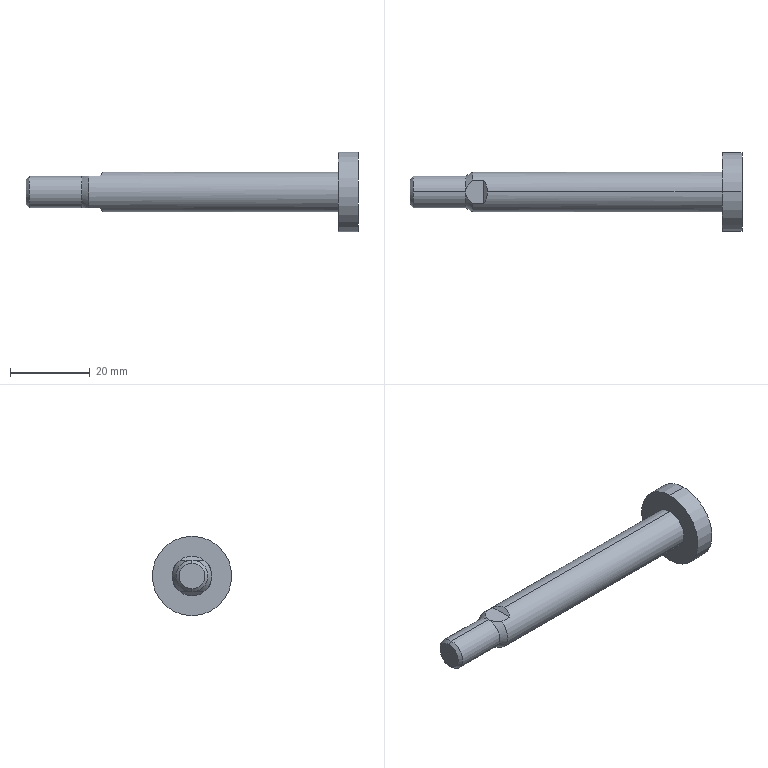Part | SolidWorks | features BaseBody 1 | 1 solid | 17 faces | box 83.5 x 20 x 20 mm | volume 7277 mm3 | plane 7 | cylinder 6 | cone 4 | commonest cylinder face diameters 8 x2 10 x2 20 x2
STEP:
#1=CARTESIAN_POINT('',(0.,3.,4.));
#2=VERTEX_POINT('',#1);
#3=CARTESIAN_POINT('',(1.,0.,5.));
#4=VERTEX_POINT('',#3);
#5=CARTESIAN_POINT('',(0.,3.,4.));
#6=CARTESIAN_POINT('',(0.6549,2.127,4.655));
#7=CARTESIAN_POINT('',(1.,1.091,5.));
#8=CARTESIAN_POINT('',(1.,0.,5.));
#9=(BOUNDED_CURVE()B_SPLINE_CURVE(3,(#5,#6,#7,#8),.UNSPECIFIED.,.F.,.T.)B_SPLINE_CURVE_WITH_KNOTS((4,4),(5.64,6.283),.UNSPECIFIED.)CURVE()GEOMETRIC_REPRESENTATION_ITEM()RATIONAL_B_SPLINE_CURVE((1.,0.9658,0.9658,1.))REPRESENTATION_ITEM(''));
#10=EDGE_CURVE('',#2,#4,#9,.T.);
#11=ORIENTED_EDGE('',*,*,#10,.T.);
#12=CARTESIAN_POINT('',(60.,0.,5.));
#13=VERTEX_POINT('',#12);
#14=CARTESIAN_POINT('',(28.616,0.,5.));
#15=DIRECTION('',(1.,0.,0.));
#16=VECTOR('',#15,1000.);
#17=LINE('',#14,#16);
#18=EDGE_CURVE('',#4,#13,#17,.T.);
#19=ORIENTED_EDGE('',*,*,#18,.T.);
#20=CARTESIAN_POINT('',(60.,0.,-5.));
#21=VERTEX_POINT('',#20);
#22=CARTESIAN_POINT('',(60.,0.,0.));
#23=DIRECTION('',(-1.,0.,0.));
#24=DIRECTION('',(0.,0.,-1.));
#25=AXIS2_PLACEMENT_3D('',#22,#23,#24);
#26=CIRCLE('',#25,5.);
#27=EDGE_CURVE('',#13,#21,#26,.T.);
#28=ORIENTED_EDGE('',*,*,#27,.T.);
#29=CARTESIAN_POINT('',(1.,0.,-5.));
#30=VERTEX_POINT('',#29);
#31=CARTESIAN_POINT('',(28.616,0.,-5.));
#32=DIRECTION('',(1.,0.,0.));
#33=VECTOR('',#32,1000.);
#34=LINE('',#31,#33);
#35=EDGE_CURVE('',#30,#21,#34,.T.);
#36=ORIENTED_EDGE('',*,*,#35,.F.);
#37=CARTESIAN_POINT('',(0.,3.,-4.));
#38=VERTEX_POINT('',#37);
#39=CARTESIAN_POINT('',(1.,0.,-5.));
#40=CARTESIAN_POINT('',(1.,1.091,-5.));
#41=CARTESIAN_POINT('',(0.6549,2.127,-4.655));
#42=CARTESIAN_POINT('',(0.,3.,-4.));
#43=(BOUNDED_CURVE()B_SPLINE_CURVE(3,(#39,#40,#41,#42),.UNSPECIFIED.,.F.,.T.)B_SPLINE_CURVE_WITH_KNOTS((4,4),(0.,0.6435),.UNSPECIFIED.)CURVE()GEOMETRIC_REPRESENTATION_ITEM()RATIONAL_B_SPLINE_CURVE((1.,0.9658,0.9658,1.))REPRESENTATION_ITEM(''));
#44=EDGE_CURVE('',#30,#38,#43,.T.);
#45=ORIENTED_EDGE('',*,*,#44,.T.);
#46=CARTESIAN_POINT('',(-2.768,3.,-4.));
#47=VERTEX_POINT('',#46);
#48=CARTESIAN_POINT('',(28.616,3.,-4.));
#49=DIRECTION('',(-1.,0.,0.));
#50=VECTOR('',#49,1000.);
#51=LINE('',#48,#50);
#52=EDGE_CURVE('',#38,#47,#51,.T.);
#53=ORIENTED_EDGE('',*,*,#52,.T.);
#54=CARTESIAN_POINT('',(-2.768,3.,4.));
#55=VERTEX_POINT('',#54);
#56=CARTESIAN_POINT('',(-2.768,0.,0.));
#57=DIRECTION('',(1.,0.,0.));
#58=DIRECTION('',(0.,0.,-1.));
#59=AXIS2_PLACEMENT_3D('',#56,#57,#58);
#60=CIRCLE('',#59,5.);
#61=EDGE_CURVE('',#47,#55,#60,.T.);
#62=ORIENTED_EDGE('',*,*,#61,.T.);
#63=CARTESIAN_POINT('',(28.616,3.,4.));
#64=DIRECTION('',(1.,0.,0.));
#65=VECTOR('',#64,1000.);
#66=LINE('',#63,#65);
#67=EDGE_CURVE('',#55,#2,#66,.T.);
#68=ORIENTED_EDGE('',*,*,#67,.T.);
#69=EDGE_LOOP('',(#11,#19,#28,#36,#45,#53,#62,#68));
#70=FACE_OUTER_BOUND('',#69,.T.);
#71=CARTESIAN_POINT('',(28.616,0.,0.));
#72=DIRECTION('',(1.,0.,0.));
#73=DIRECTION('',(0.,0.,-1.));
#74=AXIS2_PLACEMENT_3D('',#71,#72,#73);
#75=CYLINDRICAL_SURFACE('',#74,5.);
#76=ADVANCED_FACE('',(#70),#75,.T.);
#77=CARTESIAN_POINT('',(60.,0.,10.));
#78=VERTEX_POINT('',#77);
#79=CARTESIAN_POINT('',(60.,0.,-10.));
#80=VERTEX_POINT('',#79);
#81=CARTESIAN_POINT('',(60.,0.,0.));
#82=DIRECTION('',(-1.,0.,0.));
#83=DIRECTION('',(0.,0.,-1.));
#84=AXIS2_PLACEMENT_3D('',#81,#82,#83);
#85=CIRCLE('',#84,10.);
#86=EDGE_CURVE('',#78,#80,#85,.T.);
#87=ORIENTED_EDGE('',*,*,#86,.F.);
#88=CARTESIAN_POINT('',(65.,0.,10.));
#89=VERTEX_POINT('',#88);
#90=CARTESIAN_POINT('',(62.5,0.,10.));
#91=DIRECTION('',(1.,0.,0.));
#92=VECTOR('',#91,1000.);
#93=LINE('',#90,#92);
#94=EDGE_CURVE('',#78,#89,#93,.T.);
#95=ORIENTED_EDGE('',*,*,#94,.T.);
#96=CARTESIAN_POINT('',(65.,0.,-10.));
#97=VERTEX_POINT('',#96);
#98=CARTESIAN_POINT('',(65.,0.,0.));
#99=DIRECTION('',(-1.,0.,0.));
#100=DIRECTION('',(0.,0.,-1.));
#101=AXIS2_PLACEMENT_3D('',#98,#99,#100);
#102=CIRCLE('',#101,10.);
#103=EDGE_CURVE('',#89,#97,#102,.T.);
#104=ORIENTED_EDGE('',*,*,#103,.T.);
#105=CARTESIAN_POINT('',(62.5,0.,-10.));
#106=DIRECTION('',(1.,0.,0.));
#107=VECTOR('',#106,1000.);
#108=LINE('',#105,#107);
#109=EDGE_CURVE('',#80,#97,#108,.T.);
#110=ORIENTED_EDGE('',*,*,#109,.F.);
#111=EDGE_LOOP('',(#87,#95,#104,#110));
#112=FACE_OUTER_BOUND('',#111,.T.);
#113=CARTESIAN_POINT('',(62.5,0.,0.));
#114=DIRECTION('',(1.,0.,0.));
#115=DIRECTION('',(0.,0.,-1.));
#116=AXIS2_PLACEMENT_3D('',#113,#114,#115);
#117=CYLINDRICAL_SURFACE('',#116,10.);
#118=ADVANCED_FACE('',(#112),#117,.T.);
#119=CARTESIAN_POINT('',(-17.733,0.,-4.));
#120=VERTEX_POINT('',#119);
#121=CARTESIAN_POINT('',(-17.733,0.,4.));
#122=VERTEX_POINT('',#121);
#123=CARTESIAN_POINT('',(-17.733,0.,0.));
#124=DIRECTION('',(1.,0.,0.));
#125=DIRECTION('',(0.,0.,-1.));
#126=AXIS2_PLACEMENT_3D('',#123,#124,#125);
#127=CIRCLE('',#126,4.);
#128=EDGE_CURVE('',#120,#122,#127,.T.);
#129=ORIENTED_EDGE('',*,*,#128,.T.);
#130=CARTESIAN_POINT('',(-4.5,0.,4.));
#131=VERTEX_POINT('',#130);
#132=CARTESIAN_POINT('',(-11.117,0.,4.));
#133=DIRECTION('',(1.,0.,0.));
#134=VECTOR('',#133,1000.);
#135=LINE('',#132,#134);
#136=EDGE_CURVE('',#122,#131,#135,.T.);
#137=ORIENTED_EDGE('',*,*,#136,.T.);
#138=CARTESIAN_POINT('',(-4.5,0.,-4.));
#139=VERTEX_POINT('',#138);
#140=CARTESIAN_POINT('',(-4.5,0.,0.));
#141=DIRECTION('',(1.,0.,0.));
#142=DIRECTION('',(0.,1.,0.));
#143=AXIS2_PLACEMENT_3D('',#140,#141,#142);
#144=CIRCLE('',#143,4.);
#145=EDGE_CURVE('',#139,#131,#144,.T.);
#146=ORIENTED_EDGE('',*,*,#145,.F.);
#147=CARTESIAN_POINT('',(-11.117,0.,-4.));
#148=DIRECTION('',(1.,0.,0.));
#149=VECTOR('',#148,1000.);
#150=LINE('',#147,#149);
#151=EDGE_CURVE('',#120,#139,#150,.T.);
#152=ORIENTED_EDGE('',*,*,#151,.F.);
#153=EDGE_LOOP('',(#129,#137,#146,#152));
#154=FACE_OUTER_BOUND('',#153,.T.);
#155=CARTESIAN_POINT('',(-11.117,0.,0.));
#156=DIRECTION('',(1.,0.,0.));
#157=DIRECTION('',(0.,0.,-1.));
#158=AXIS2_PLACEMENT_3D('',#155,#156,#157);
#159=CYLINDRICAL_SURFACE('',#158,4.);
#160=ADVANCED_FACE('',(#154),#159,.T.);
#161=CARTESIAN_POINT('',(-18.5,0.,-3.233));
#162=VERTEX_POINT('',#161);
#163=CARTESIAN_POINT('',(-18.5,0.,3.233));
#164=VERTEX_POINT('',#163);
#165=CARTESIAN_POINT('',(-18.5,0.,0.));
#166=DIRECTION('',(1.,0.,0.));
#167=DIRECTION('',(0.,0.,-1.));
#168=AXIS2_PLACEMENT_3D('',#165,#166,#167);
#169=CIRCLE('',#168,3.233);
#170=EDGE_CURVE('',#162,#164,#169,.T.);
#171=ORIENTED_EDGE('',*,*,#170,.T.);
#172=CARTESIAN_POINT('',(-17.733,0.,4.));
#173=DIRECTION('',(0.7071,0.,0.7071));
#174=VECTOR('',#173,1000.);
#175=LINE('',#172,#174);
#176=EDGE_CURVE('',#164,#122,#175,.T.);
#177=ORIENTED_EDGE('',*,*,#176,.T.);
#178=ORIENTED_EDGE('',*,*,#128,.F.);
#179=CARTESIAN_POINT('',(-17.733,0.,-4.));
#180=DIRECTION('',(0.7071,0.,-0.7071));
#181=VECTOR('',#180,1000.);
#182=LINE('',#179,#181);
#183=EDGE_CURVE('',#162,#120,#182,.T.);
#184=ORIENTED_EDGE('',*,*,#183,.F.);
#185=EDGE_LOOP('',(#171,#177,#178,#184));
#186=FACE_OUTER_BOUND('',#185,.T.);
#187=CARTESIAN_POINT('',(-17.733,0.,0.));
#188=DIRECTION('',(1.,0.,0.));
#189=DIRECTION('',(0.,0.,-1.));
#190=AXIS2_PLACEMENT_3D('',#187,#188,#189);
#191=CONICAL_SURFACE('',#190,4.,0.7854);
#192=ADVANCED_FACE('',(#186),#191,.T.);
#193=ORIENTED_EDGE('',*,*,#18,.F.);
#194=CARTESIAN_POINT('',(0.,-3.,4.));
#195=VERTEX_POINT('',#194);
#196=CARTESIAN_POINT('',(1.,0.,5.));
#197=CARTESIAN_POINT('',(1.,-1.091,5.));
#198=CARTESIAN_POINT('',(0.6549,-2.127,4.655));
#199=CARTESIAN_POINT('',(0.,-3.,4.));
#200=(BOUNDED_CURVE()B_SPLINE_CURVE(3,(#196,#197,#198,#199),.UNSPECIFIED.,.F.,.T.)B_SPLINE_CURVE_WITH_KNOTS((4,4),(0.,0.6435),.UNSPECIFIED.)CURVE()GEOMETRIC_REPRESENTATION_ITEM()RATIONAL_B_SPLINE_CURVE((1.,0.9658,0.9658,1.))REPRESENTATION_ITEM(''));
#201=EDGE_CURVE('',#4,#195,#200,.T.);
#202=ORIENTED_EDGE('',*,*,#201,.T.);
#203=CARTESIAN_POINT('',(-2.768,-3.,4.));
#204=VERTEX_POINT('',#203);
#205=CARTESIAN_POINT('',(28.616,-3.,4.));
#206=DIRECTION('',(-1.,0.,0.));
#207=VECTOR('',#206,1000.);
#208=LINE('',#205,#207);
#209=EDGE_CURVE('',#195,#204,#208,.T.);
#210=ORIENTED_EDGE('',*,*,#209,.T.);
#211=CARTESIAN_POINT('',(-2.768,-3.,-4.));
#212=VERTEX_POINT('',#211);
#213=CARTESIAN_POINT('',(-2.768,0.,0.));
#214=DIRECTION('',(1.,0.,0.));
#215=DIRECTION('',(0.,0.,-1.));
#216=AXIS2_PLACEMENT_3D('',#213,#214,#215);
#217=CIRCLE('',#216,5.);
#218=EDGE_CURVE('',#204,#212,#217,.T.);
#219=ORIENTED_EDGE('',*,*,#218,.T.);
#220=CARTESIAN_POINT('',(0.,-3.,-4.));
#221=VERTEX_POINT('',#220);
#222=CARTESIAN_POINT('',(28.616,-3.,-4.));
#223=DIRECTION('',(1.,0.,0.));
#224=VECTOR('',#223,1000.);
#225=LINE('',#222,#224);
#226=EDGE_CURVE('',#212,#221,#225,.T.);
#227=ORIENTED_EDGE('',*,*,#226,.T.);
#228=CARTESIAN_POINT('',(0.,-3.,-4.));
#229=CARTESIAN_POINT('',(0.6549,-2.127,-4.655));
#230=CARTESIAN_POINT('',(1.,-1.091,-5.));
#231=CARTESIAN_POINT('',(1.,0.,-5.));
#232=(BOUNDED_CURVE()B_SPLINE_CURVE(3,(#228,#229,#230,#231),.UNSPECIFIED.,.F.,.T.)B_SPLINE_CURVE_WITH_KNOTS((4,4),(5.64,6.283),.UNSPECIFIED.)CURVE()GEOMETRIC_REPRESENTATION_ITEM()RATIONAL_B_SPLINE_CURVE((1.,0.9658,0.9658,1.))REPRESENTATION_ITEM(''));
#233=EDGE_CURVE('',#221,#30,#232,.T.);
#234=ORIENTED_EDGE('',*,*,#233,.T.);
#235=ORIENTED_EDGE('',*,*,#35,.T.);
#236=CARTESIAN_POINT('',(60.,0.,0.));
#237=DIRECTION('',(-1.,0.,0.));
#238=DIRECTION('',(0.,0.,-1.));
#239=AXIS2_PLACEMENT_3D('',#236,#237,#238);
#240=CIRCLE('',#239,5.);
#241=EDGE_CURVE('',#21,#13,#240,.T.);
#242=ORIENTED_EDGE('',*,*,#241,.T.);
#243=EDGE_LOOP('',(#193,#202,#210,#219,#227,#234,#235,#242));
#244=FACE_OUTER_BOUND('',#243,.T.);
#245=CARTESIAN_POINT('',(28.616,0.,0.));
#246=DIRECTION('',(1.,0.,0.));
#247=DIRECTION('',(0.,0.,-1.));
#248=AXIS2_PLACEMENT_3D('',#245,#246,#247);
#249=CYLINDRICAL_SURFACE('',#248,5.);
#250=ADVANCED_FACE('',(#244),#249,.T.);
#251=CARTESIAN_POINT('',(60.,0.,0.));
#252=DIRECTION('',(-1.,0.,0.));
#253=DIRECTION('',(0.,0.,-1.));
#254=AXIS2_PLACEMENT_3D('',#251,#252,#253);
#255=CIRCLE('',#254,10.);
#256=EDGE_CURVE('',#80,#78,#255,.T.);
#257=ORIENTED_EDGE('',*,*,#256,.T.);
#258=ORIENTED_EDGE('',*,*,#86,.T.);
#259=EDGE_LOOP('',(#257,#258));
#260=FACE_OUTER_BOUND('',#259,.T.);
#261=ORIENTED_EDGE('',*,*,#241,.F.);
#262=ORIENTED_EDGE('',*,*,#27,.F.);
#263=EDGE_LOOP('',(#261,#262));
#264=FACE_BOUND('',#263,.T.);
#265=CARTESIAN_POINT('',(60.,7.5,0.));
#266=DIRECTION('',(-1.,0.,0.));
#267=DIRECTION('',(0.,0.,1.));
#268=AXIS2_PLACEMENT_3D('',#265,#266,#267);
#269=PLANE('',#268);
#270=ADVANCED_FACE('',(#260,#264),#269,.T.);
#271=CARTESIAN_POINT('',(-2.768,-3.,4.));
#272=CARTESIAN_POINT('',(-2.982,-2.794,4.));
#273=CARTESIAN_POINT('',(-3.188,-2.582,4.));
#274=CARTESIAN_POINT('',(-3.579,-2.139,4.));
#275=CARTESIAN_POINT('',(-3.763,-1.908,4.));
#276=CARTESIAN_POINT('',(-4.092,-1.412,4.));
#277=CARTESIAN_POINT('',(-4.234,-1.151,4.));
#278=CARTESIAN_POINT('',(-4.388,-0.7338,4.));
#279=CARTESIAN_POINT('',(-4.43,-0.589,4.));
#280=CARTESIAN_POINT('',(-4.485,-0.2975,4.));
#281=CARTESIAN_POINT('',(-4.5,-0.1498,4.));
#282=CARTESIAN_POINT('',(-4.5,0.,4.));
#283=B_SPLINE_CURVE_WITH_KNOTS('',3,(#271,#272,#273,#274,#275,#276,#277,#278,#279,#280,#281,#282),.UNSPECIFIED.,.F.,.F.,(4,2,2,2,2,4),(0.,0.0008859,0.001772,0.002658,0.0031,0.003543),.UNSPECIFIED.);
#284=EDGE_CURVE('',#204,#131,#283,.T.);
#285=ORIENTED_EDGE('',*,*,#284,.T.);
#286=CARTESIAN_POINT('',(-4.5,0.,0.));
#287=DIRECTION('',(1.,0.,0.));
#288=DIRECTION('',(0.,1.,0.));
#289=AXIS2_PLACEMENT_3D('',#286,#287,#288);
#290=CIRCLE('',#289,4.);
#291=EDGE_CURVE('',#131,#139,#290,.T.);
#292=ORIENTED_EDGE('',*,*,#291,.T.);
#293=CARTESIAN_POINT('',(-4.5,0.,-4.));
#294=CARTESIAN_POINT('',(-4.5,-0.3003,-4.));
#295=CARTESIAN_POINT('',(-4.441,-0.5891,-4.));
#296=CARTESIAN_POINT('',(-4.235,-1.149,-4.));
#297=CARTESIAN_POINT('',(-4.093,-1.41,-4.));
#298=CARTESIAN_POINT('',(-3.767,-1.902,-4.));
#299=CARTESIAN_POINT('',(-3.581,-2.136,-4.));
#300=CARTESIAN_POINT('',(-3.189,-2.581,-4.));
#301=CARTESIAN_POINT('',(-2.982,-2.794,-4.));
#302=CARTESIAN_POINT('',(-2.768,-3.,-4.));
#303=B_SPLINE_CURVE_WITH_KNOTS('',3,(#293,#294,#295,#296,#297,#298,#299,#300,#301,#302),.UNSPECIFIED.,.F.,.F.,(4,2,2,2,4),(0.,0.0008841,0.001768,0.002652,0.003536),.UNSPECIFIED.);
#304=EDGE_CURVE('',#139,#212,#303,.T.);
#305=ORIENTED_EDGE('',*,*,#304,.T.);
#306=ORIENTED_EDGE('',*,*,#218,.F.);
#307=EDGE_LOOP('',(#285,#292,#305,#306));
#308=FACE_OUTER_BOUND('',#307,.T.);
#309=CARTESIAN_POINT('',(-2.768,0.,0.));
#310=DIRECTION('',(1.,0.,0.));
#311=DIRECTION('',(0.,0.,-1.));
#312=AXIS2_PLACEMENT_3D('',#309,#310,#311);
#313=CONICAL_SURFACE('',#312,5.,0.5236);
#314=ADVANCED_FACE('',(#308),#313,.T.);
#315=CARTESIAN_POINT('',(0.,10.,4.));
#316=DIRECTION('',(0.,-1.,0.));
#317=VECTOR('',#316,1000.);
#318=LINE('',#315,#317);
#319=EDGE_CURVE('',#2,#195,#318,.T.);
#320=ORIENTED_EDGE('',*,*,#319,.F.);
#321=ORIENTED_EDGE('',*,*,#67,.F.);
#322=CARTESIAN_POINT('',(-4.5,0.,4.));
#323=CARTESIAN_POINT('',(-4.5,0.3003,4.));
#324=CARTESIAN_POINT('',(-4.441,0.5891,4.));
#325=CARTESIAN_POINT('',(-4.235,1.149,4.));
#326=CARTESIAN_POINT('',(-4.093,1.41,4.));
#327=CARTESIAN_POINT('',(-3.767,1.902,4.));
#328=CARTESIAN_POINT('',(-3.581,2.136,4.));
#329=CARTESIAN_POINT('',(-3.189,2.581,4.));
#330=CARTESIAN_POINT('',(-2.982,2.794,4.));
#331=CARTESIAN_POINT('',(-2.768,3.,4.));
#332=B_SPLINE_CURVE_WITH_KNOTS('',3,(#322,#323,#324,#325,#326,#327,#328,#329,#330,#331),.UNSPECIFIED.,.F.,.F.,(4,2,2,2,4),(0.,0.0008841,0.001768,0.002652,0.003536),.UNSPECIFIED.);
#333=EDGE_CURVE('',#131,#55,#332,.T.);
#334=ORIENTED_EDGE('',*,*,#333,.F.);
#335=ORIENTED_EDGE('',*,*,#284,.F.);
#336=ORIENTED_EDGE('',*,*,#209,.F.);
#337=EDGE_LOOP('',(#320,#321,#334,#335,#336));
#338=FACE_OUTER_BOUND('',#337,.T.);
#339=CARTESIAN_POINT('',(0.,10.,4.));
#340=DIRECTION('',(0.,0.,-1.));
#341=DIRECTION('',(-1.,0.,0.));
#342=AXIS2_PLACEMENT_3D('',#339,#340,#341);
#343=PLANE('',#342);
#344=ADVANCED_FACE('',(#338),#343,.F.);
#345=ORIENTED_EDGE('',*,*,#319,.T.);
#346=ORIENTED_EDGE('',*,*,#201,.F.);
#347=ORIENTED_EDGE('',*,*,#10,.F.);
#348=EDGE_LOOP('',(#345,#346,#347));
#349=FACE_OUTER_BOUND('',#348,.T.);
#350=CARTESIAN_POINT('',(5.,10.,9.));
#351=DIRECTION('',(0.7071,0.,-0.7071));
#352=DIRECTION('',(-0.7071,0.,-0.7071));
#353=AXIS2_PLACEMENT_3D('',#350,#351,#352);
#354=PLANE('',#353);
#355=ADVANCED_FACE('',(#349),#354,.F.);
#356=ORIENTED_EDGE('',*,*,#333,.T.);
#357=ORIENTED_EDGE('',*,*,#61,.F.);
#358=CARTESIAN_POINT('',(-2.768,3.,-4.));
#359=CARTESIAN_POINT('',(-2.982,2.794,-4.));
#360=CARTESIAN_POINT('',(-3.188,2.582,-4.));
#361=CARTESIAN_POINT('',(-3.579,2.139,-4.));
#362=CARTESIAN_POINT('',(-3.763,1.908,-4.));
#363=CARTESIAN_POINT('',(-4.092,1.412,-4.));
#364=CARTESIAN_POINT('',(-4.234,1.151,-4.));
#365=CARTESIAN_POINT('',(-4.388,0.7338,-4.));
#366=CARTESIAN_POINT('',(-4.43,0.589,-4.));
#367=CARTESIAN_POINT('',(-4.485,0.2975,-4.));
#368=CARTESIAN_POINT('',(-4.5,0.1498,-4.));
#369=CARTESIAN_POINT('',(-4.5,0.,-4.));
#370=B_SPLINE_CURVE_WITH_KNOTS('',3,(#358,#359,#360,#361,#362,#363,#364,#365,#366,#367,#368,#369),.UNSPECIFIED.,.F.,.F.,(4,2,2,2,2,4),(0.,0.0008859,0.001772,0.002658,0.0031,0.003543),.UNSPECIFIED.);
#371=EDGE_CURVE('',#47,#139,#370,.T.);
#372=ORIENTED_EDGE('',*,*,#371,.T.);
#373=ORIENTED_EDGE('',*,*,#145,.T.);
#374=EDGE_LOOP('',(#356,#357,#372,#373));
#375=FACE_OUTER_BOUND('',#374,.T.);
#376=CARTESIAN_POINT('',(-2.768,0.,0.));
#377=DIRECTION('',(1.,0.,0.));
#378=DIRECTION('',(0.,0.,-1.));
#379=AXIS2_PLACEMENT_3D('',#376,#377,#378);
#380=CONICAL_SURFACE('',#379,5.,0.5236);
#381=ADVANCED_FACE('',(#375),#380,.T.);
#382=ORIENTED_EDGE('',*,*,#94,.F.);
#383=ORIENTED_EDGE('',*,*,#256,.F.);
#384=ORIENTED_EDGE('',*,*,#109,.T.);
#385=CARTESIAN_POINT('',(65.,0.,0.));
#386=DIRECTION('',(-1.,0.,0.));
#387=DIRECTION('',(0.,0.,-1.));
#388=AXIS2_PLACEMENT_3D('',#385,#386,#387);
#389=CIRCLE('',#388,10.);
#390=EDGE_CURVE('',#97,#89,#389,.T.);
#391=ORIENTED_EDGE('',*,*,#390,.T.);
#392=EDGE_LOOP('',(#382,#383,#384,#391));
#393=FACE_OUTER_BOUND('',#392,.T.);
#394=CARTESIAN_POINT('',(62.5,0.,0.));
#395=DIRECTION('',(1.,0.,0.));
#396=DIRECTION('',(0.,0.,-1.));
#397=AXIS2_PLACEMENT_3D('',#394,#395,#396);
#398=CYLINDRICAL_SURFACE('',#397,10.);
#399=ADVANCED_FACE('',(#393),#398,.T.);
#400=CARTESIAN_POINT('',(0.,10.,-4.));
#401=DIRECTION('',(0.,1.,0.));
#402=VECTOR('',#401,1000.);
#403=LINE('',#400,#402);
#404=EDGE_CURVE('',#221,#38,#403,.T.);
#405=ORIENTED_EDGE('',*,*,#404,.F.);
#406=ORIENTED_EDGE('',*,*,#226,.F.);
#407=ORIENTED_EDGE('',*,*,#304,.F.);
#408=ORIENTED_EDGE('',*,*,#371,.F.);
#409=ORIENTED_EDGE('',*,*,#52,.F.);
#410=EDGE_LOOP('',(#405,#406,#407,#408,#409));
#411=FACE_OUTER_BOUND('',#410,.T.);
#412=CARTESIAN_POINT('',(-4.5,10.,-4.));
#413=DIRECTION('',(0.,0.,1.));
#414=DIRECTION('',(1.,0.,0.));
#415=AXIS2_PLACEMENT_3D('',#412,#413,#414);
#416=PLANE('',#415);
#417=ADVANCED_FACE('',(#411),#416,.F.);
#418=ORIENTED_EDGE('',*,*,#404,.T.);
#419=ORIENTED_EDGE('',*,*,#44,.F.);
#420=ORIENTED_EDGE('',*,*,#233,.F.);
#421=EDGE_LOOP('',(#418,#419,#420));
#422=FACE_OUTER_BOUND('',#421,.T.);
#423=CARTESIAN_POINT('',(0.,10.,-4.));
#424=DIRECTION('',(0.7071,0.,0.7071));
#425=DIRECTION('',(0.7071,0.,-0.7071));
#426=AXIS2_PLACEMENT_3D('',#423,#424,#425);
#427=PLANE('',#426);
#428=ADVANCED_FACE('',(#422),#427,.F.);
#429=ORIENTED_EDGE('',*,*,#136,.F.);
#430=CARTESIAN_POINT('',(-17.733,0.,0.));
#431=DIRECTION('',(1.,0.,0.));
#432=DIRECTION('',(0.,0.,-1.));
#433=AXIS2_PLACEMENT_3D('',#430,#431,#432);
#434=CIRCLE('',#433,4.);
#435=EDGE_CURVE('',#122,#120,#434,.T.);
#436=ORIENTED_EDGE('',*,*,#435,.T.);
#437=ORIENTED_EDGE('',*,*,#151,.T.);
#438=ORIENTED_EDGE('',*,*,#291,.F.);
#439=EDGE_LOOP('',(#429,#436,#437,#438));
#440=FACE_OUTER_BOUND('',#439,.T.);
#441=CARTESIAN_POINT('',(-11.117,0.,0.));
#442=DIRECTION('',(1.,0.,0.));
#443=DIRECTION('',(0.,0.,-1.));
#444=AXIS2_PLACEMENT_3D('',#441,#442,#443);
#445=CYLINDRICAL_SURFACE('',#444,4.);
#446=ADVANCED_FACE('',(#440),#445,.T.);
#447=ORIENTED_EDGE('',*,*,#390,.F.);
#448=ORIENTED_EDGE('',*,*,#103,.F.);
#449=EDGE_LOOP('',(#447,#448));
#450=FACE_OUTER_BOUND('',#449,.T.);
#451=CARTESIAN_POINT('',(65.,5.,0.));
#452=DIRECTION('',(1.,0.,0.));
#453=DIRECTION('',(0.,0.,-1.));
#454=AXIS2_PLACEMENT_3D('',#451,#452,#453);
#455=PLANE('',#454);
#456=ADVANCED_FACE('',(#450),#455,.T.);
#457=ORIENTED_EDGE('',*,*,#176,.F.);
#458=CARTESIAN_POINT('',(-18.5,0.,0.));
#459=DIRECTION('',(1.,0.,0.));
#460=DIRECTION('',(0.,0.,-1.));
#461=AXIS2_PLACEMENT_3D('',#458,#459,#460);
#462=CIRCLE('',#461,3.233);
#463=EDGE_CURVE('',#164,#162,#462,.T.);
#464=ORIENTED_EDGE('',*,*,#463,.T.);
#465=ORIENTED_EDGE('',*,*,#183,.T.);
#466=ORIENTED_EDGE('',*,*,#435,.F.);
#467=EDGE_LOOP('',(#457,#464,#465,#466));
#468=FACE_OUTER_BOUND('',#467,.T.);
#469=CARTESIAN_POINT('',(-17.733,0.,0.));
#470=DIRECTION('',(1.,0.,0.));
#471=DIRECTION('',(0.,0.,-1.));
#472=AXIS2_PLACEMENT_3D('',#469,#470,#471);
#473=CONICAL_SURFACE('',#472,4.,0.7854);
#474=ADVANCED_FACE('',(#468),#473,.T.);
#475=ORIENTED_EDGE('',*,*,#170,.F.);
#476=ORIENTED_EDGE('',*,*,#463,.F.);
#477=EDGE_LOOP('',(#475,#476));
#478=FACE_OUTER_BOUND('',#477,.T.);
#479=CARTESIAN_POINT('',(-18.5,1.617,0.));
#480=DIRECTION('',(-1.,0.,0.));
#481=DIRECTION('',(0.,0.,1.));
#482=AXIS2_PLACEMENT_3D('',#479,#480,#481);
#483=PLANE('',#482);
#484=ADVANCED_FACE('',(#478),#483,.T.);
#485=CLOSED_SHELL('',(#76,#118,#160,#192,#250,#270,#314,#344,#355,#381,#399,#417,#428,#446,#456,#474,#484));
#486=MANIFOLD_SOLID_BREP('',#485);
#487=CARTESIAN_POINT('',(0.,0.,0.));
#488=DIRECTION('',(0.,0.,1.));
#489=DIRECTION('',(1.,0.,0.));
#490=AXIS2_PLACEMENT_3D('',#487,#488,#489);
#491=(LENGTH_UNIT()NAMED_UNIT(*)SI_UNIT(.MILLI.,.METRE.));
#492=UNCERTAINTY_MEASURE_WITH_UNIT(LENGTH_MEASURE(0.00001),#491,'','');
#493=(NAMED_UNIT(*)PLANE_ANGLE_UNIT()SI_UNIT($,.RADIAN.));
#494=(NAMED_UNIT(*)SI_UNIT($,.STERADIAN.)SOLID_ANGLE_UNIT());
#495=(GEOMETRIC_REPRESENTATION_CONTEXT(3)GLOBAL_UNCERTAINTY_ASSIGNED_CONTEXT((#492))GLOBAL_UNIT_ASSIGNED_CONTEXT((#491,#493,#494))REPRESENTATION_CONTEXT('',''));
#496=ADVANCED_BREP_SHAPE_REPRESENTATION('',(#486,#490),#495);